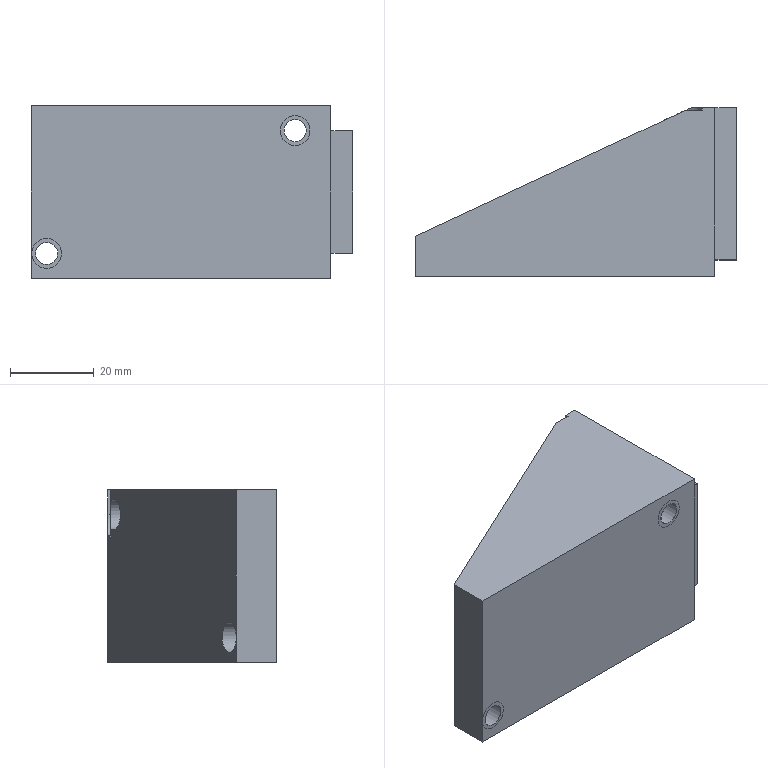Part | STEP file | 4-20.sldasm-Part-179 | 1 solid | 24 faces | box 76.9 x 40.4 x 41.3 mm | volume 81109 mm3 | plane 15 | cylinder 9 | commonest cylinder face diameters 5.319 x4 7.142 x4 11.112 x1
STEP:
#1=CARTESIAN_POINT('',(270.795,574.024,-96.871));
#2=VERTEX_POINT('',#1);
#3=CARTESIAN_POINT('',(270.795,574.024,-89.729));
#4=VERTEX_POINT('',#3);
#5=CARTESIAN_POINT('',(270.795,574.024,-96.871));
#6=CARTESIAN_POINT('',(263.653,570.694,-96.871));
#7=CARTESIAN_POINT('',(263.653,570.694,-89.729));
#8=CARTESIAN_POINT('',(270.795,574.024,-89.729));
#9=(BOUNDED_CURVE()B_SPLINE_CURVE(3,(#5,#6,#7,#8),.UNSPECIFIED.,.F.,.F.)B_SPLINE_CURVE_WITH_KNOTS((4,4),(4.712,7.854),.UNSPECIFIED.)CURVE()GEOMETRIC_REPRESENTATION_ITEM()RATIONAL_B_SPLINE_CURVE((1.,0.3333,0.3333,1.))REPRESENTATION_ITEM(''));
#10=EDGE_CURVE('',#2,#4,#9,.T.);
#11=ORIENTED_EDGE('',*,*,#10,.T.);
#12=CARTESIAN_POINT('',(270.795,535.064,-89.729));
#13=VERTEX_POINT('',#12);
#14=CARTESIAN_POINT('',(270.795,574.688,-89.729));
#15=DIRECTION('',(0.,-1.,0.));
#16=VECTOR('',#15,1000.);
#17=LINE('',#14,#16);
#18=EDGE_CURVE('',#4,#13,#17,.T.);
#19=ORIENTED_EDGE('',*,*,#18,.T.);
#20=CARTESIAN_POINT('',(270.795,535.064,-96.871));
#21=VERTEX_POINT('',#20);
#22=CARTESIAN_POINT('',(270.795,535.064,-93.3));
#23=DIRECTION('',(0.,1.,0.));
#24=DIRECTION('',(0.,0.,-1.));
#25=AXIS2_PLACEMENT_3D('',#22,#23,#24);
#26=CIRCLE('',#25,3.571);
#27=EDGE_CURVE('',#21,#13,#26,.T.);
#28=ORIENTED_EDGE('',*,*,#27,.F.);
#29=CARTESIAN_POINT('',(270.795,574.688,-96.871));
#30=DIRECTION('',(0.,-1.,0.));
#31=VECTOR('',#30,1000.);
#32=LINE('',#29,#31);
#33=EDGE_CURVE('',#2,#21,#32,.T.);
#34=ORIENTED_EDGE('',*,*,#33,.F.);
#35=EDGE_LOOP('',(#11,#19,#28,#34));
#36=FACE_OUTER_BOUND('',#35,.T.);
#37=CARTESIAN_POINT('',(270.795,574.688,-93.3));
#38=DIRECTION('',(0.,-1.,0.));
#39=DIRECTION('',(0.,0.,-1.));
#40=AXIS2_PLACEMENT_3D('',#37,#38,#39);
#41=CYLINDRICAL_SURFACE('',#40,3.571);
#42=ADVANCED_FACE('',(#36),#41,.F.);
#43=CARTESIAN_POINT('',(270.795,535.064,-95.959));
#44=VERTEX_POINT('',#43);
#45=CARTESIAN_POINT('',(270.795,535.064,-90.641));
#46=VERTEX_POINT('',#45);
#47=CARTESIAN_POINT('',(270.795,535.064,-93.3));
#48=DIRECTION('',(0.,1.,0.));
#49=DIRECTION('',(0.,0.,-1.));
#50=AXIS2_PLACEMENT_3D('',#47,#48,#49);
#51=CIRCLE('',#50,2.659);
#52=EDGE_CURVE('',#44,#46,#51,.T.);
#53=ORIENTED_EDGE('',*,*,#52,.T.);
#54=CARTESIAN_POINT('',(270.795,535.,-90.641));
#55=VERTEX_POINT('',#54);
#56=CARTESIAN_POINT('',(270.795,574.688,-90.641));
#57=DIRECTION('',(0.,-1.,0.));
#58=VECTOR('',#57,1000.);
#59=LINE('',#56,#58);
#60=EDGE_CURVE('',#46,#55,#59,.T.);
#61=ORIENTED_EDGE('',*,*,#60,.T.);
#62=CARTESIAN_POINT('',(270.795,535.,-95.959));
#63=VERTEX_POINT('',#62);
#64=CARTESIAN_POINT('',(270.795,535.,-93.3));
#65=DIRECTION('',(0.,1.,0.));
#66=DIRECTION('',(0.,0.,1.));
#67=AXIS2_PLACEMENT_3D('',#64,#65,#66);
#68=CIRCLE('',#67,2.659);
#69=EDGE_CURVE('',#63,#55,#68,.T.);
#70=ORIENTED_EDGE('',*,*,#69,.F.);
#71=CARTESIAN_POINT('',(270.795,574.688,-95.959));
#72=DIRECTION('',(0.,-1.,0.));
#73=VECTOR('',#72,1000.);
#74=LINE('',#71,#73);
#75=EDGE_CURVE('',#44,#63,#74,.T.);
#76=ORIENTED_EDGE('',*,*,#75,.F.);
#77=EDGE_LOOP('',(#53,#61,#70,#76));
#78=FACE_OUTER_BOUND('',#77,.T.);
#79=CARTESIAN_POINT('',(270.795,574.688,-93.3));
#80=DIRECTION('',(0.,-1.,0.));
#81=DIRECTION('',(0.,0.,-1.));
#82=AXIS2_PLACEMENT_3D('',#79,#80,#81);
#83=CYLINDRICAL_SURFACE('',#82,2.659);
#84=ADVANCED_FACE('',(#78),#83,.F.);
#85=CARTESIAN_POINT('',(211.295,546.279,-119.129));
#86=VERTEX_POINT('',#85);
#87=CARTESIAN_POINT('',(211.295,546.279,-126.271));
#88=VERTEX_POINT('',#87);
#89=CARTESIAN_POINT('',(211.295,546.279,-119.129));
#90=CARTESIAN_POINT('',(218.438,549.61,-119.129));
#91=CARTESIAN_POINT('',(218.438,549.61,-126.271));
#92=CARTESIAN_POINT('',(211.295,546.279,-126.271));
#93=(BOUNDED_CURVE()B_SPLINE_CURVE(3,(#89,#90,#91,#92),.UNSPECIFIED.,.F.,.F.)B_SPLINE_CURVE_WITH_KNOTS((4,4),(1.571,4.712),.UNSPECIFIED.)CURVE()GEOMETRIC_REPRESENTATION_ITEM()RATIONAL_B_SPLINE_CURVE((1.,0.3333,0.3333,1.))REPRESENTATION_ITEM(''));
#94=EDGE_CURVE('',#86,#88,#93,.T.);
#95=ORIENTED_EDGE('',*,*,#94,.T.);
#96=CARTESIAN_POINT('',(211.295,535.064,-126.271));
#97=VERTEX_POINT('',#96);
#98=CARTESIAN_POINT('',(211.295,574.688,-126.271));
#99=DIRECTION('',(0.,-1.,0.));
#100=VECTOR('',#99,1000.);
#101=LINE('',#98,#100);
#102=EDGE_CURVE('',#88,#97,#101,.T.);
#103=ORIENTED_EDGE('',*,*,#102,.T.);
#104=CARTESIAN_POINT('',(211.295,535.064,-119.129));
#105=VERTEX_POINT('',#104);
#106=CARTESIAN_POINT('',(211.295,535.064,-122.7));
#107=DIRECTION('',(0.,-1.,0.));
#108=DIRECTION('',(0.,0.,1.));
#109=AXIS2_PLACEMENT_3D('',#106,#107,#108);
#110=CIRCLE('',#109,3.571);
#111=EDGE_CURVE('',#97,#105,#110,.T.);
#112=ORIENTED_EDGE('',*,*,#111,.T.);
#113=CARTESIAN_POINT('',(211.295,574.688,-119.129));
#114=DIRECTION('',(0.,-1.,0.));
#115=VECTOR('',#114,1000.);
#116=LINE('',#113,#115);
#117=EDGE_CURVE('',#86,#105,#116,.T.);
#118=ORIENTED_EDGE('',*,*,#117,.F.);
#119=EDGE_LOOP('',(#95,#103,#112,#118));
#120=FACE_OUTER_BOUND('',#119,.T.);
#121=CARTESIAN_POINT('',(211.295,574.688,-122.7));
#122=DIRECTION('',(0.,-1.,0.));
#123=DIRECTION('',(0.,0.,1.));
#124=AXIS2_PLACEMENT_3D('',#121,#122,#123);
#125=CYLINDRICAL_SURFACE('',#124,3.571);
#126=ADVANCED_FACE('',(#120),#125,.F.);
#127=CARTESIAN_POINT('',(211.295,535.064,-125.359));
#128=VERTEX_POINT('',#127);
#129=CARTESIAN_POINT('',(211.295,535.064,-120.041));
#130=VERTEX_POINT('',#129);
#131=CARTESIAN_POINT('',(211.295,535.064,-122.7));
#132=DIRECTION('',(0.,-1.,0.));
#133=DIRECTION('',(0.,0.,1.));
#134=AXIS2_PLACEMENT_3D('',#131,#132,#133);
#135=CIRCLE('',#134,2.659);
#136=EDGE_CURVE('',#128,#130,#135,.T.);
#137=ORIENTED_EDGE('',*,*,#136,.F.);
#138=CARTESIAN_POINT('',(211.295,535.,-125.359));
#139=VERTEX_POINT('',#138);
#140=CARTESIAN_POINT('',(211.295,574.688,-125.359));
#141=DIRECTION('',(0.,-1.,0.));
#142=VECTOR('',#141,1000.);
#143=LINE('',#140,#142);
#144=EDGE_CURVE('',#128,#139,#143,.T.);
#145=ORIENTED_EDGE('',*,*,#144,.T.);
#146=CARTESIAN_POINT('',(211.295,535.,-120.041));
#147=VERTEX_POINT('',#146);
#148=CARTESIAN_POINT('',(211.295,535.,-122.7));
#149=DIRECTION('',(0.,1.,0.));
#150=DIRECTION('',(0.,0.,1.));
#151=AXIS2_PLACEMENT_3D('',#148,#149,#150);
#152=CIRCLE('',#151,2.659);
#153=EDGE_CURVE('',#147,#139,#152,.T.);
#154=ORIENTED_EDGE('',*,*,#153,.F.);
#155=CARTESIAN_POINT('',(211.295,574.688,-120.041));
#156=DIRECTION('',(0.,-1.,0.));
#157=VECTOR('',#156,1000.);
#158=LINE('',#155,#157);
#159=EDGE_CURVE('',#130,#147,#158,.T.);
#160=ORIENTED_EDGE('',*,*,#159,.F.);
#161=EDGE_LOOP('',(#137,#145,#154,#160));
#162=FACE_OUTER_BOUND('',#161,.T.);
#163=CARTESIAN_POINT('',(211.295,574.688,-122.7));
#164=DIRECTION('',(0.,-1.,0.));
#165=DIRECTION('',(0.,0.,1.));
#166=AXIS2_PLACEMENT_3D('',#163,#164,#165);
#167=CYLINDRICAL_SURFACE('',#166,2.659);
#168=ADVANCED_FACE('',(#162),#167,.F.);
#169=CARTESIAN_POINT('',(276.351,574.688,-93.3));
#170=VERTEX_POINT('',#169);
#171=CARTESIAN_POINT('',(276.351,575.4,-93.3));
#172=VERTEX_POINT('',#171);
#173=CARTESIAN_POINT('',(276.351,578.244,-93.3));
#174=DIRECTION('',(0.,1.,0.));
#175=VECTOR('',#174,1000.);
#176=LINE('',#173,#175);
#177=EDGE_CURVE('',#170,#172,#176,.T.);
#178=ORIENTED_EDGE('',*,*,#177,.T.);
#179=CARTESIAN_POINT('',(273.745,575.4,-98.008));
#180=VERTEX_POINT('',#179);
#181=CARTESIAN_POINT('',(270.795,575.4,-93.3));
#182=DIRECTION('',(0.,1.,0.));
#183=DIRECTION('',(0.,0.,-1.));
#184=AXIS2_PLACEMENT_3D('',#181,#182,#183);
#185=CIRCLE('',#184,5.556);
#186=EDGE_CURVE('',#172,#180,#185,.T.);
#187=ORIENTED_EDGE('',*,*,#186,.T.);
#188=CARTESIAN_POINT('',(272.218,574.688,-98.671));
#189=VERTEX_POINT('',#188);
#190=CARTESIAN_POINT('',(273.745,575.4,-98.008));
#191=CARTESIAN_POINT('',(273.271,575.179,-98.305));
#192=CARTESIAN_POINT('',(272.759,574.94,-98.528));
#193=CARTESIAN_POINT('',(272.218,574.688,-98.671));
#194=(BOUNDED_CURVE()B_SPLINE_CURVE(3,(#190,#191,#192,#193),.UNSPECIFIED.,.F.,.F.)B_SPLINE_CURVE_WITH_KNOTS((4,4),(1.011,1.312),.UNSPECIFIED.)CURVE()GEOMETRIC_REPRESENTATION_ITEM()RATIONAL_B_SPLINE_CURVE((1.,0.9925,0.9925,1.))REPRESENTATION_ITEM(''));
#195=EDGE_CURVE('',#180,#189,#194,.T.);
#196=ORIENTED_EDGE('',*,*,#195,.T.);
#197=CARTESIAN_POINT('',(270.795,574.688,-93.3));
#198=DIRECTION('',(0.,-1.,0.));
#199=DIRECTION('',(0.,0.,1.));
#200=AXIS2_PLACEMENT_3D('',#197,#198,#199);
#201=CIRCLE('',#200,5.556);
#202=EDGE_CURVE('',#189,#170,#201,.T.);
#203=ORIENTED_EDGE('',*,*,#202,.T.);
#204=EDGE_LOOP('',(#178,#187,#196,#203));
#205=FACE_OUTER_BOUND('',#204,.T.);
#206=CARTESIAN_POINT('',(270.795,574.688,-93.3));
#207=DIRECTION('',(0.,1.,0.));
#208=DIRECTION('',(0.,0.,1.));
#209=AXIS2_PLACEMENT_3D('',#206,#207,#208);
#210=CYLINDRICAL_SURFACE('',#209,5.556);
#211=ADVANCED_FACE('',(#205),#210,.F.);
#212=ORIENTED_EDGE('',*,*,#153,.T.);
#213=CARTESIAN_POINT('',(211.295,535.,-122.7));
#214=DIRECTION('',(0.,1.,0.));
#215=DIRECTION('',(0.,0.,1.));
#216=AXIS2_PLACEMENT_3D('',#213,#214,#215);
#217=CIRCLE('',#216,2.659);
#218=EDGE_CURVE('',#139,#147,#217,.T.);
#219=ORIENTED_EDGE('',*,*,#218,.T.);
#220=EDGE_LOOP('',(#212,#219));
#221=FACE_BOUND('',#220,.T.);
#222=CARTESIAN_POINT('',(279.345,535.,-128.65));
#223=VERTEX_POINT('',#222);
#224=CARTESIAN_POINT('',(279.345,535.,-87.35));
#225=VERTEX_POINT('',#224);
#226=CARTESIAN_POINT('',(279.345,535.,-128.65));
#227=DIRECTION('',(0.,0.,1.));
#228=VECTOR('',#227,1000.);
#229=LINE('',#226,#228);
#230=EDGE_CURVE('',#223,#225,#229,.T.);
#231=ORIENTED_EDGE('',*,*,#230,.T.);
#232=CARTESIAN_POINT('',(207.645,535.,-87.35));
#233=VERTEX_POINT('',#232);
#234=CARTESIAN_POINT('',(246.645,535.,-87.35));
#235=DIRECTION('',(-1.,0.,0.));
#236=VECTOR('',#235,1000.);
#237=LINE('',#234,#236);
#238=EDGE_CURVE('',#225,#233,#237,.T.);
#239=ORIENTED_EDGE('',*,*,#238,.T.);
#240=CARTESIAN_POINT('',(207.645,535.,-128.65));
#241=VERTEX_POINT('',#240);
#242=CARTESIAN_POINT('',(207.645,535.,-128.65));
#243=DIRECTION('',(0.,0.,1.));
#244=VECTOR('',#243,1000.);
#245=LINE('',#242,#244);
#246=EDGE_CURVE('',#241,#233,#245,.T.);
#247=ORIENTED_EDGE('',*,*,#246,.F.);
#248=CARTESIAN_POINT('',(246.645,535.,-128.65));
#249=DIRECTION('',(1.,0.,0.));
#250=VECTOR('',#249,1000.);
#251=LINE('',#248,#250);
#252=EDGE_CURVE('',#241,#223,#251,.T.);
#253=ORIENTED_EDGE('',*,*,#252,.T.);
#254=EDGE_LOOP('',(#231,#239,#247,#253));
#255=FACE_OUTER_BOUND('',#254,.T.);
#256=ORIENTED_EDGE('',*,*,#69,.T.);
#257=CARTESIAN_POINT('',(270.795,535.,-93.3));
#258=DIRECTION('',(0.,1.,0.));
#259=DIRECTION('',(0.,0.,1.));
#260=AXIS2_PLACEMENT_3D('',#257,#258,#259);
#261=CIRCLE('',#260,2.659);
#262=EDGE_CURVE('',#55,#63,#261,.T.);
#263=ORIENTED_EDGE('',*,*,#262,.T.);
#264=EDGE_LOOP('',(#256,#263));
#265=FACE_BOUND('',#264,.T.);
#266=CARTESIAN_POINT('',(246.645,535.,-128.65));
#267=DIRECTION('',(0.,-1.,0.));
#268=DIRECTION('',(0.,0.,1.));
#269=AXIS2_PLACEMENT_3D('',#266,#267,#268);
#270=PLANE('',#269);
#271=ADVANCED_FACE('',(#221,#255,#265),#270,.T.);
#272=CARTESIAN_POINT('',(276.351,574.688,-87.35));
#273=VERTEX_POINT('',#272);
#274=CARTESIAN_POINT('',(276.351,575.4,-87.35));
#275=VERTEX_POINT('',#274);
#276=CARTESIAN_POINT('',(276.351,555.2,-87.35));
#277=DIRECTION('',(0.,1.,0.));
#278=VECTOR('',#277,1000.);
#279=LINE('',#276,#278);
#280=EDGE_CURVE('',#273,#275,#279,.T.);
#281=ORIENTED_EDGE('',*,*,#280,.F.);
#282=CARTESIAN_POINT('',(272.218,574.688,-87.35));
#283=VERTEX_POINT('',#282);
#284=CARTESIAN_POINT('',(246.645,574.688,-87.35));
#285=DIRECTION('',(1.,0.,0.));
#286=VECTOR('',#285,1000.);
#287=LINE('',#284,#286);
#288=EDGE_CURVE('',#283,#273,#287,.T.);
#289=ORIENTED_EDGE('',*,*,#288,.F.);
#290=CARTESIAN_POINT('',(207.645,544.577,-87.35));
#291=VERTEX_POINT('',#290);
#292=CARTESIAN_POINT('',(243.748,561.412,-87.35));
#293=DIRECTION('',(-0.9063,-0.4226,0.));
#294=VECTOR('',#293,1000.);
#295=LINE('',#292,#294);
#296=EDGE_CURVE('',#283,#291,#295,.T.);
#297=ORIENTED_EDGE('',*,*,#296,.T.);
#298=CARTESIAN_POINT('',(207.645,555.2,-87.35));
#299=DIRECTION('',(0.,1.,0.));
#300=VECTOR('',#299,1000.);
#301=LINE('',#298,#300);
#302=EDGE_CURVE('',#233,#291,#301,.T.);
#303=ORIENTED_EDGE('',*,*,#302,.F.);
#304=ORIENTED_EDGE('',*,*,#238,.F.);
#305=CARTESIAN_POINT('',(279.345,575.4,-87.35));
#306=VERTEX_POINT('',#305);
#307=CARTESIAN_POINT('',(279.345,555.2,-87.35));
#308=DIRECTION('',(0.,-1.,0.));
#309=VECTOR('',#308,1000.);
#310=LINE('',#307,#309);
#311=EDGE_CURVE('',#306,#225,#310,.T.);
#312=ORIENTED_EDGE('',*,*,#311,.F.);
#313=CARTESIAN_POINT('',(246.645,575.4,-87.35));
#314=DIRECTION('',(1.,0.,0.));
#315=VECTOR('',#314,1000.);
#316=LINE('',#313,#315);
#317=EDGE_CURVE('',#275,#306,#316,.T.);
#318=ORIENTED_EDGE('',*,*,#317,.F.);
#319=EDGE_LOOP('',(#281,#289,#297,#303,#304,#312,#318));
#320=FACE_OUTER_BOUND('',#319,.T.);
#321=CARTESIAN_POINT('',(246.645,555.2,-87.35));
#322=DIRECTION('',(0.,0.,1.));
#323=DIRECTION('',(0.,1.,0.));
#324=AXIS2_PLACEMENT_3D('',#321,#322,#323);
#325=PLANE('',#324);
#326=ADVANCED_FACE('',(#320),#325,.T.);
#327=CARTESIAN_POINT('',(279.345,575.4,-93.3));
#328=VERTEX_POINT('',#327);
#329=CARTESIAN_POINT('',(279.345,538.9,-93.3));
#330=VERTEX_POINT('',#329);
#331=CARTESIAN_POINT('',(279.345,555.2,-93.3));
#332=DIRECTION('',(0.,-1.,0.));
#333=VECTOR('',#332,1000.);
#334=LINE('',#331,#333);
#335=EDGE_CURVE('',#328,#330,#334,.T.);
#336=ORIENTED_EDGE('',*,*,#335,.F.);
#337=CARTESIAN_POINT('',(279.345,575.4,-128.65));
#338=DIRECTION('',(0.,0.,1.));
#339=VECTOR('',#338,1000.);
#340=LINE('',#337,#339);
#341=EDGE_CURVE('',#328,#306,#340,.T.);
#342=ORIENTED_EDGE('',*,*,#341,.T.);
#343=ORIENTED_EDGE('',*,*,#311,.T.);
#344=ORIENTED_EDGE('',*,*,#230,.F.);
#345=CARTESIAN_POINT('',(279.345,575.4,-128.65));
#346=VERTEX_POINT('',#345);
#347=CARTESIAN_POINT('',(279.345,555.2,-128.65));
#348=DIRECTION('',(0.,1.,0.));
#349=VECTOR('',#348,1000.);
#350=LINE('',#347,#349);
#351=EDGE_CURVE('',#223,#346,#350,.T.);
#352=ORIENTED_EDGE('',*,*,#351,.T.);
#353=CARTESIAN_POINT('',(279.345,575.4,-122.7));
#354=VERTEX_POINT('',#353);
#355=CARTESIAN_POINT('',(279.345,575.4,-128.65));
#356=DIRECTION('',(0.,0.,1.));
#357=VECTOR('',#356,1000.);
#358=LINE('',#355,#357);
#359=EDGE_CURVE('',#346,#354,#358,.T.);
#360=ORIENTED_EDGE('',*,*,#359,.T.);
#361=CARTESIAN_POINT('',(279.345,538.9,-122.7));
#362=VERTEX_POINT('',#361);
#363=CARTESIAN_POINT('',(279.345,555.2,-122.7));
#364=DIRECTION('',(0.,1.,0.));
#365=VECTOR('',#364,1000.);
#366=LINE('',#363,#365);
#367=EDGE_CURVE('',#362,#354,#366,.T.);
#368=ORIENTED_EDGE('',*,*,#367,.F.);
#369=CARTESIAN_POINT('',(279.345,538.9,-108.));
#370=DIRECTION('',(0.,0.,1.));
#371=VECTOR('',#370,1000.);
#372=LINE('',#369,#371);
#373=EDGE_CURVE('',#362,#330,#372,.T.);
#374=ORIENTED_EDGE('',*,*,#373,.T.);
#375=EDGE_LOOP('',(#336,#342,#343,#344,#352,#360,#368,#374));
#376=FACE_OUTER_BOUND('',#375,.T.);
#377=CARTESIAN_POINT('',(279.345,555.2,-128.65));
#378=DIRECTION('',(1.,0.,0.));
#379=DIRECTION('',(0.,0.,-1.));
#380=AXIS2_PLACEMENT_3D('',#377,#378,#379);
#381=PLANE('',#380);
#382=ADVANCED_FACE('',(#376),#381,.T.);
#383=ORIENTED_EDGE('',*,*,#302,.T.);
#384=CARTESIAN_POINT('',(207.645,544.577,-128.65));
#385=VERTEX_POINT('',#384);
#386=CARTESIAN_POINT('',(207.645,544.577,-128.65));
#387=DIRECTION('',(0.,0.,-1.));
#388=VECTOR('',#387,1000.);
#389=LINE('',#386,#388);
#390=EDGE_CURVE('',#291,#385,#389,.T.);
#391=ORIENTED_EDGE('',*,*,#390,.T.);
#392=CARTESIAN_POINT('',(207.645,555.2,-128.65));
#393=DIRECTION('',(0.,-1.,0.));
#394=VECTOR('',#393,1000.);
#395=LINE('',#392,#394);
#396=EDGE_CURVE('',#385,#241,#395,.T.);
#397=ORIENTED_EDGE('',*,*,#396,.T.);
#398=ORIENTED_EDGE('',*,*,#246,.T.);
#399=EDGE_LOOP('',(#383,#391,#397,#398));
#400=FACE_OUTER_BOUND('',#399,.T.);
#401=CARTESIAN_POINT('',(207.645,555.2,-128.65));
#402=DIRECTION('',(-1.,0.,0.));
#403=DIRECTION('',(0.,0.,1.));
#404=AXIS2_PLACEMENT_3D('',#401,#402,#403);
#405=PLANE('',#404);
#406=ADVANCED_FACE('',(#400),#405,.T.);
#407=ORIENTED_EDGE('',*,*,#396,.F.);
#408=CARTESIAN_POINT('',(273.745,575.4,-128.65));
#409=VERTEX_POINT('',#408);
#410=CARTESIAN_POINT('',(243.748,561.412,-128.65));
#411=DIRECTION('',(0.9063,0.4226,0.));
#412=VECTOR('',#411,1000.);
#413=LINE('',#410,#412);
#414=EDGE_CURVE('',#385,#409,#413,.T.);
#415=ORIENTED_EDGE('',*,*,#414,.T.);
#416=CARTESIAN_POINT('',(246.645,575.4,-128.65));
#417=DIRECTION('',(-1.,0.,0.));
#418=VECTOR('',#417,1000.);
#419=LINE('',#416,#418);
#420=EDGE_CURVE('',#346,#409,#419,.T.);
#421=ORIENTED_EDGE('',*,*,#420,.F.);
#422=ORIENTED_EDGE('',*,*,#351,.F.);
#423=ORIENTED_EDGE('',*,*,#252,.F.);
#424=EDGE_LOOP('',(#407,#415,#421,#422,#423));
#425=FACE_OUTER_BOUND('',#424,.T.);
#426=CARTESIAN_POINT('',(246.645,555.2,-128.65));
#427=DIRECTION('',(0.,0.,-1.));
#428=DIRECTION('',(0.,-1.,0.));
#429=AXIS2_PLACEMENT_3D('',#426,#427,#428);
#430=PLANE('',#429);
#431=ADVANCED_FACE('',(#425),#430,.T.);
#432=CARTESIAN_POINT('',(276.351,575.4,-128.65));
#433=DIRECTION('',(0.,0.,-1.));
#434=VECTOR('',#433,1000.);
#435=LINE('',#432,#434);
#436=EDGE_CURVE('',#275,#172,#435,.T.);
#437=ORIENTED_EDGE('',*,*,#436,.F.);
#438=ORIENTED_EDGE('',*,*,#317,.T.);
#439=ORIENTED_EDGE('',*,*,#341,.F.);
#440=CARTESIAN_POINT('',(284.545,575.4,-93.3));
#441=VERTEX_POINT('',#440);
#442=CARTESIAN_POINT('',(307.945,575.4,-93.3));
#443=DIRECTION('',(-1.,0.,0.));
#444=VECTOR('',#443,1000.);
#445=LINE('',#442,#444);
#446=EDGE_CURVE('',#441,#328,#445,.T.);
#447=ORIENTED_EDGE('',*,*,#446,.F.);
#448=CARTESIAN_POINT('',(284.545,575.4,-122.7));
#449=VERTEX_POINT('',#448);
#450=CARTESIAN_POINT('',(284.545,575.4,-128.65));
#451=DIRECTION('',(0.,0.,1.));
#452=VECTOR('',#451,1000.);
#453=LINE('',#450,#452);
#454=EDGE_CURVE('',#449,#441,#453,.T.);
#455=ORIENTED_EDGE('',*,*,#454,.F.);
#456=CARTESIAN_POINT('',(307.945,575.4,-122.7));
#457=DIRECTION('',(-1.,0.,0.));
#458=VECTOR('',#457,1000.);
#459=LINE('',#456,#458);
#460=EDGE_CURVE('',#449,#354,#459,.T.);
#461=ORIENTED_EDGE('',*,*,#460,.T.);
#462=ORIENTED_EDGE('',*,*,#359,.F.);
#463=ORIENTED_EDGE('',*,*,#420,.T.);
#464=CARTESIAN_POINT('',(273.745,575.4,-128.65));
#465=DIRECTION('',(0.,0.,1.));
#466=VECTOR('',#465,1000.);
#467=LINE('',#464,#466);
#468=EDGE_CURVE('',#409,#180,#467,.T.);
#469=ORIENTED_EDGE('',*,*,#468,.T.);
#470=ORIENTED_EDGE('',*,*,#186,.F.);
#471=EDGE_LOOP('',(#437,#438,#439,#447,#455,#461,#462,#463,#469,#470));
#472=FACE_OUTER_BOUND('',#471,.T.);
#473=CARTESIAN_POINT('',(246.645,575.4,-128.65));
#474=DIRECTION('',(0.,1.,0.));
#475=DIRECTION('',(0.,0.,-1.));
#476=AXIS2_PLACEMENT_3D('',#473,#474,#475);
#477=PLANE('',#476);
#478=ADVANCED_FACE('',(#472),#477,.T.);
#479=ORIENTED_EDGE('',*,*,#296,.F.);
#480=CARTESIAN_POINT('',(272.218,574.688,-90.025));
#481=VERTEX_POINT('',#480);
#482=CARTESIAN_POINT('',(272.218,574.688,-128.65));
#483=DIRECTION('',(0.,0.,1.));
#484=VECTOR('',#483,1000.);
#485=LINE('',#482,#484);
#486=EDGE_CURVE('',#481,#283,#485,.T.);
#487=ORIENTED_EDGE('',*,*,#486,.F.);
#488=CARTESIAN_POINT('',(270.795,574.024,-89.729));
#489=CARTESIAN_POINT('',(271.286,574.254,-89.729));
#490=CARTESIAN_POINT('',(271.767,574.478,-89.829));
#491=CARTESIAN_POINT('',(272.218,574.688,-90.025));
#492=(BOUNDED_CURVE()B_SPLINE_CURVE(3,(#488,#489,#490,#491),.UNSPECIFIED.,.F.,.F.)B_SPLINE_CURVE_WITH_KNOTS((4,4),(1.571,1.981),.UNSPECIFIED.)CURVE()GEOMETRIC_REPRESENTATION_ITEM()RATIONAL_B_SPLINE_CURVE((1.,0.986,0.986,1.))REPRESENTATION_ITEM(''));
#493=EDGE_CURVE('',#4,#481,#492,.T.);
#494=ORIENTED_EDGE('',*,*,#493,.F.);
#495=ORIENTED_EDGE('',*,*,#10,.F.);
#496=CARTESIAN_POINT('',(272.218,574.688,-96.575));
#497=VERTEX_POINT('',#496);
#498=CARTESIAN_POINT('',(272.218,574.688,-96.575));
#499=CARTESIAN_POINT('',(271.767,574.478,-96.771));
#500=CARTESIAN_POINT('',(271.286,574.254,-96.871));
#501=CARTESIAN_POINT('',(270.795,574.024,-96.871));
#502=(BOUNDED_CURVE()B_SPLINE_CURVE(3,(#498,#499,#500,#501),.UNSPECIFIED.,.F.,.F.)B_SPLINE_CURVE_WITH_KNOTS((4,4),(4.303,4.712),.UNSPECIFIED.)CURVE()GEOMETRIC_REPRESENTATION_ITEM()RATIONAL_B_SPLINE_CURVE((1.,0.986,0.986,1.))REPRESENTATION_ITEM(''));
#503=EDGE_CURVE('',#497,#2,#502,.T.);
#504=ORIENTED_EDGE('',*,*,#503,.F.);
#505=CARTESIAN_POINT('',(272.218,574.688,-128.65));
#506=DIRECTION('',(0.,0.,1.));
#507=VECTOR('',#506,1000.);
#508=LINE('',#505,#507);
#509=EDGE_CURVE('',#189,#497,#508,.T.);
#510=ORIENTED_EDGE('',*,*,#509,.F.);
#511=ORIENTED_EDGE('',*,*,#195,.F.);
#512=ORIENTED_EDGE('',*,*,#468,.F.);
#513=ORIENTED_EDGE('',*,*,#414,.F.);
#514=ORIENTED_EDGE('',*,*,#390,.F.);
#515=EDGE_LOOP('',(#479,#487,#494,#495,#504,#510,#511,#512,#513,#514));
#516=FACE_OUTER_BOUND('',#515,.T.);
#517=ORIENTED_EDGE('',*,*,#94,.F.);
#518=CARTESIAN_POINT('',(211.295,546.279,-126.271));
#519=CARTESIAN_POINT('',(204.153,542.948,-126.271));
#520=CARTESIAN_POINT('',(204.153,542.948,-119.129));
#521=CARTESIAN_POINT('',(211.295,546.279,-119.129));
#522=(BOUNDED_CURVE()B_SPLINE_CURVE(3,(#518,#519,#520,#521),.UNSPECIFIED.,.F.,.F.)B_SPLINE_CURVE_WITH_KNOTS((4,4),(4.712,7.854),.UNSPECIFIED.)CURVE()GEOMETRIC_REPRESENTATION_ITEM()RATIONAL_B_SPLINE_CURVE((1.,0.3333,0.3333,1.))REPRESENTATION_ITEM(''));
#523=EDGE_CURVE('',#88,#86,#522,.T.);
#524=ORIENTED_EDGE('',*,*,#523,.F.);
#525=EDGE_LOOP('',(#517,#524));
#526=FACE_BOUND('',#525,.T.);
#527=CARTESIAN_POINT('',(273.745,575.4,-128.65));
#528=DIRECTION('',(0.4226,-0.9063,0.));
#529=DIRECTION('',(0.9063,0.4226,0.));
#530=AXIS2_PLACEMENT_3D('',#527,#528,#529);
#531=PLANE('',#530);
#532=ADVANCED_FACE('',(#516,#526),#531,.F.);
#533=ORIENTED_EDGE('',*,*,#144,.F.);
#534=CARTESIAN_POINT('',(211.295,535.064,-122.7));
#535=DIRECTION('',(0.,-1.,0.));
#536=DIRECTION('',(0.,0.,1.));
#537=AXIS2_PLACEMENT_3D('',#534,#535,#536);
#538=CIRCLE('',#537,2.659);
#539=EDGE_CURVE('',#130,#128,#538,.T.);
#540=ORIENTED_EDGE('',*,*,#539,.F.);
#541=ORIENTED_EDGE('',*,*,#159,.T.);
#542=ORIENTED_EDGE('',*,*,#218,.F.);
#543=EDGE_LOOP('',(#533,#540,#541,#542));
#544=FACE_OUTER_BOUND('',#543,.T.);
#545=CARTESIAN_POINT('',(211.295,574.688,-122.7));
#546=DIRECTION('',(0.,-1.,0.));
#547=DIRECTION('',(0.,0.,1.));
#548=AXIS2_PLACEMENT_3D('',#545,#546,#547);
#549=CYLINDRICAL_SURFACE('',#548,2.659);
#550=ADVANCED_FACE('',(#544),#549,.F.);
#551=CARTESIAN_POINT('',(211.295,535.064,-122.7));
#552=DIRECTION('',(0.,-1.,0.));
#553=DIRECTION('',(0.,0.,1.));
#554=AXIS2_PLACEMENT_3D('',#551,#552,#553);
#555=CIRCLE('',#554,3.571);
#556=EDGE_CURVE('',#105,#97,#555,.T.);
#557=ORIENTED_EDGE('',*,*,#556,.F.);
#558=ORIENTED_EDGE('',*,*,#111,.F.);
#559=EDGE_LOOP('',(#557,#558));
#560=FACE_OUTER_BOUND('',#559,.T.);
#561=ORIENTED_EDGE('',*,*,#539,.T.);
#562=ORIENTED_EDGE('',*,*,#136,.T.);
#563=EDGE_LOOP('',(#561,#562));
#564=FACE_BOUND('',#563,.T.);
#565=CARTESIAN_POINT('',(211.295,535.064,-122.7));
#566=DIRECTION('',(0.,-1.,0.));
#567=DIRECTION('',(0.,0.,1.));
#568=AXIS2_PLACEMENT_3D('',#565,#566,#567);
#569=PLANE('',#568);
#570=ADVANCED_FACE('',(#560,#564),#569,.F.);
#571=ORIENTED_EDGE('',*,*,#102,.F.);
#572=ORIENTED_EDGE('',*,*,#523,.T.);
#573=ORIENTED_EDGE('',*,*,#117,.T.);
#574=ORIENTED_EDGE('',*,*,#556,.T.);
#575=EDGE_LOOP('',(#571,#572,#573,#574));
#576=FACE_OUTER_BOUND('',#575,.T.);
#577=CARTESIAN_POINT('',(211.295,574.688,-122.7));
#578=DIRECTION('',(0.,-1.,0.));
#579=DIRECTION('',(0.,0.,1.));
#580=AXIS2_PLACEMENT_3D('',#577,#578,#579);
#581=CYLINDRICAL_SURFACE('',#580,3.571);
#582=ADVANCED_FACE('',(#576),#581,.F.);
#583=ORIENTED_EDGE('',*,*,#60,.F.);
#584=CARTESIAN_POINT('',(270.795,535.064,-93.3));
#585=DIRECTION('',(0.,1.,0.));
#586=DIRECTION('',(0.,0.,-1.));
#587=AXIS2_PLACEMENT_3D('',#584,#585,#586);
#588=CIRCLE('',#587,2.659);
#589=EDGE_CURVE('',#46,#44,#588,.T.);
#590=ORIENTED_EDGE('',*,*,#589,.T.);
#591=ORIENTED_EDGE('',*,*,#75,.T.);
#592=ORIENTED_EDGE('',*,*,#262,.F.);
#593=EDGE_LOOP('',(#583,#590,#591,#592));
#594=FACE_OUTER_BOUND('',#593,.T.);
#595=CARTESIAN_POINT('',(270.795,574.688,-93.3));
#596=DIRECTION('',(0.,-1.,0.));
#597=DIRECTION('',(0.,0.,-1.));
#598=AXIS2_PLACEMENT_3D('',#595,#596,#597);
#599=CYLINDRICAL_SURFACE('',#598,2.659);
#600=ADVANCED_FACE('',(#594),#599,.F.);
#601=ORIENTED_EDGE('',*,*,#27,.T.);
#602=CARTESIAN_POINT('',(270.795,535.064,-93.3));
#603=DIRECTION('',(0.,1.,0.));
#604=DIRECTION('',(0.,0.,-1.));
#605=AXIS2_PLACEMENT_3D('',#602,#603,#604);
#606=CIRCLE('',#605,3.571);
#607=EDGE_CURVE('',#13,#21,#606,.T.);
#608=ORIENTED_EDGE('',*,*,#607,.T.);
#609=EDGE_LOOP('',(#601,#608));
#610=FACE_OUTER_BOUND('',#609,.T.);
#611=ORIENTED_EDGE('',*,*,#52,.F.);
#612=ORIENTED_EDGE('',*,*,#589,.F.);
#613=EDGE_LOOP('',(#611,#612));
#614=FACE_BOUND('',#613,.T.);
#615=CARTESIAN_POINT('',(270.795,535.064,-93.3));
#616=DIRECTION('',(0.,-1.,0.));
#617=DIRECTION('',(0.,0.,-1.));
#618=AXIS2_PLACEMENT_3D('',#615,#616,#617);
#619=PLANE('',#618);
#620=ADVANCED_FACE('',(#610,#614),#619,.F.);
#621=ORIENTED_EDGE('',*,*,#18,.F.);
#622=ORIENTED_EDGE('',*,*,#493,.T.);
#623=CARTESIAN_POINT('',(270.795,574.688,-93.3));
#624=DIRECTION('',(0.,1.,0.));
#625=DIRECTION('',(0.,0.,-1.));
#626=AXIS2_PLACEMENT_3D('',#623,#624,#625);
#627=CIRCLE('',#626,3.571);
#628=EDGE_CURVE('',#481,#497,#627,.T.);
#629=ORIENTED_EDGE('',*,*,#628,.T.);
#630=ORIENTED_EDGE('',*,*,#503,.T.);
#631=ORIENTED_EDGE('',*,*,#33,.T.);
#632=ORIENTED_EDGE('',*,*,#607,.F.);
#633=EDGE_LOOP('',(#621,#622,#629,#630,#631,#632));
#634=FACE_OUTER_BOUND('',#633,.T.);
#635=CARTESIAN_POINT('',(270.795,574.688,-93.3));
#636=DIRECTION('',(0.,-1.,0.));
#637=DIRECTION('',(0.,0.,-1.));
#638=AXIS2_PLACEMENT_3D('',#635,#636,#637);
#639=CYLINDRICAL_SURFACE('',#638,3.571);
#640=ADVANCED_FACE('',(#634),#639,.F.);
#641=ORIENTED_EDGE('',*,*,#509,.T.);
#642=ORIENTED_EDGE('',*,*,#628,.F.);
#643=ORIENTED_EDGE('',*,*,#486,.T.);
#644=ORIENTED_EDGE('',*,*,#288,.T.);
#645=CARTESIAN_POINT('',(276.351,574.688,-98.856));
#646=DIRECTION('',(0.,0.,1.));
#647=VECTOR('',#646,1000.);
#648=LINE('',#645,#647);
#649=EDGE_CURVE('',#170,#273,#648,.T.);
#650=ORIENTED_EDGE('',*,*,#649,.F.);
#651=ORIENTED_EDGE('',*,*,#202,.F.);
#652=EDGE_LOOP('',(#641,#642,#643,#644,#650,#651));
#653=FACE_OUTER_BOUND('',#652,.T.);
#654=CARTESIAN_POINT('',(270.795,574.688,-93.3));
#655=DIRECTION('',(0.,-1.,0.));
#656=DIRECTION('',(0.,0.,-1.));
#657=AXIS2_PLACEMENT_3D('',#654,#655,#656);
#658=PLANE('',#657);
#659=ADVANCED_FACE('',(#653),#658,.F.);
#660=CARTESIAN_POINT('',(284.545,538.9,-122.7));
#661=VERTEX_POINT('',#660);
#662=CARTESIAN_POINT('',(307.945,538.9,-122.7));
#663=DIRECTION('',(-1.,0.,0.));
#664=VECTOR('',#663,1000.);
#665=LINE('',#662,#664);
#666=EDGE_CURVE('',#661,#362,#665,.T.);
#667=ORIENTED_EDGE('',*,*,#666,.F.);
#668=CARTESIAN_POINT('',(284.545,538.9,-93.3));
#669=VERTEX_POINT('',#668);
#670=CARTESIAN_POINT('',(284.545,538.9,-108.));
#671=DIRECTION('',(0.,0.,1.));
#672=VECTOR('',#671,1000.);
#673=LINE('',#670,#672);
#674=EDGE_CURVE('',#661,#669,#673,.T.);
#675=ORIENTED_EDGE('',*,*,#674,.T.);
#676=CARTESIAN_POINT('',(307.945,538.9,-93.3));
#677=DIRECTION('',(-1.,0.,0.));
#678=VECTOR('',#677,1000.);
#679=LINE('',#676,#678);
#680=EDGE_CURVE('',#669,#330,#679,.T.);
#681=ORIENTED_EDGE('',*,*,#680,.T.);
#682=ORIENTED_EDGE('',*,*,#373,.F.);
#683=EDGE_LOOP('',(#667,#675,#681,#682));
#684=FACE_OUTER_BOUND('',#683,.T.);
#685=CARTESIAN_POINT('',(307.945,538.9,-108.));
#686=DIRECTION('',(0.,-1.,0.));
#687=DIRECTION('',(0.,0.,1.));
#688=AXIS2_PLACEMENT_3D('',#685,#686,#687);
#689=PLANE('',#688);
#690=ADVANCED_FACE('',(#684),#689,.T.);
#691=CARTESIAN_POINT('',(284.545,555.2,-93.3));
#692=DIRECTION('',(0.,-1.,0.));
#693=VECTOR('',#692,1000.);
#694=LINE('',#691,#693);
#695=EDGE_CURVE('',#441,#669,#694,.T.);
#696=ORIENTED_EDGE('',*,*,#695,.F.);
#697=ORIENTED_EDGE('',*,*,#446,.T.);
#698=ORIENTED_EDGE('',*,*,#335,.T.);
#699=ORIENTED_EDGE('',*,*,#680,.F.);
#700=EDGE_LOOP('',(#696,#697,#698,#699));
#701=FACE_OUTER_BOUND('',#700,.T.);
#702=CARTESIAN_POINT('',(307.945,555.2,-93.3));
#703=DIRECTION('',(0.,0.,-1.));
#704=DIRECTION('',(0.,-1.,0.));
#705=AXIS2_PLACEMENT_3D('',#702,#703,#704);
#706=PLANE('',#705);
#707=ADVANCED_FACE('',(#701),#706,.F.);
#708=CARTESIAN_POINT('',(284.545,555.2,-122.7));
#709=DIRECTION('',(0.,1.,0.));
#710=VECTOR('',#709,1000.);
#711=LINE('',#708,#710);
#712=EDGE_CURVE('',#661,#449,#711,.T.);
#713=ORIENTED_EDGE('',*,*,#712,.F.);
#714=ORIENTED_EDGE('',*,*,#666,.T.);
#715=ORIENTED_EDGE('',*,*,#367,.T.);
#716=ORIENTED_EDGE('',*,*,#460,.F.);
#717=EDGE_LOOP('',(#713,#714,#715,#716));
#718=FACE_OUTER_BOUND('',#717,.T.);
#719=CARTESIAN_POINT('',(307.945,555.2,-122.7));
#720=DIRECTION('',(0.,0.,1.));
#721=DIRECTION('',(0.,1.,0.));
#722=AXIS2_PLACEMENT_3D('',#719,#720,#721);
#723=PLANE('',#722);
#724=ADVANCED_FACE('',(#718),#723,.F.);
#725=ORIENTED_EDGE('',*,*,#674,.F.);
#726=ORIENTED_EDGE('',*,*,#712,.T.);
#727=ORIENTED_EDGE('',*,*,#454,.T.);
#728=ORIENTED_EDGE('',*,*,#695,.T.);
#729=EDGE_LOOP('',(#725,#726,#727,#728));
#730=FACE_OUTER_BOUND('',#729,.T.);
#731=CARTESIAN_POINT('',(284.545,535.,-108.));
#732=DIRECTION('',(1.,0.,0.));
#733=DIRECTION('',(0.,-1.,0.));
#734=AXIS2_PLACEMENT_3D('',#731,#732,#733);
#735=PLANE('',#734);
#736=ADVANCED_FACE('',(#730),#735,.T.);
#737=ORIENTED_EDGE('',*,*,#280,.T.);
#738=ORIENTED_EDGE('',*,*,#436,.T.);
#739=ORIENTED_EDGE('',*,*,#177,.F.);
#740=ORIENTED_EDGE('',*,*,#649,.T.);
#741=EDGE_LOOP('',(#737,#738,#739,#740));
#742=FACE_OUTER_BOUND('',#741,.T.);
#743=CARTESIAN_POINT('',(276.351,578.244,-98.856));
#744=DIRECTION('',(1.,0.,0.));
#745=DIRECTION('',(0.,0.,-1.));
#746=AXIS2_PLACEMENT_3D('',#743,#744,#745);
#747=PLANE('',#746);
#748=ADVANCED_FACE('',(#742),#747,.F.);
#749=CLOSED_SHELL('',(#42,#84,#126,#168,#211,#271,#326,#382,#406,#431,#478,#532,#550,#570,#582,#600,#620,#640,#659,#690,#707,#724,#736,#748));
#750=MANIFOLD_SOLID_BREP('',#749);
#751=CARTESIAN_POINT('',(0.,0.,0.));
#752=DIRECTION('',(0.,0.,1.));
#753=DIRECTION('',(1.,0.,0.));
#754=AXIS2_PLACEMENT_3D('',#751,#752,#753);
#755=(LENGTH_UNIT()NAMED_UNIT(*)SI_UNIT(.MILLI.,.METRE.));
#756=UNCERTAINTY_MEASURE_WITH_UNIT(LENGTH_MEASURE(0.00001),#755,'','');
#757=(NAMED_UNIT(*)PLANE_ANGLE_UNIT()SI_UNIT($,.RADIAN.));
#758=(NAMED_UNIT(*)SI_UNIT($,.STERADIAN.)SOLID_ANGLE_UNIT());
#759=(GEOMETRIC_REPRESENTATION_CONTEXT(3)GLOBAL_UNCERTAINTY_ASSIGNED_CONTEXT((#756))GLOBAL_UNIT_ASSIGNED_CONTEXT((#755,#757,#758))REPRESENTATION_CONTEXT('',''));
#760=ADVANCED_BREP_SHAPE_REPRESENTATION('',(#750,#754),#759);